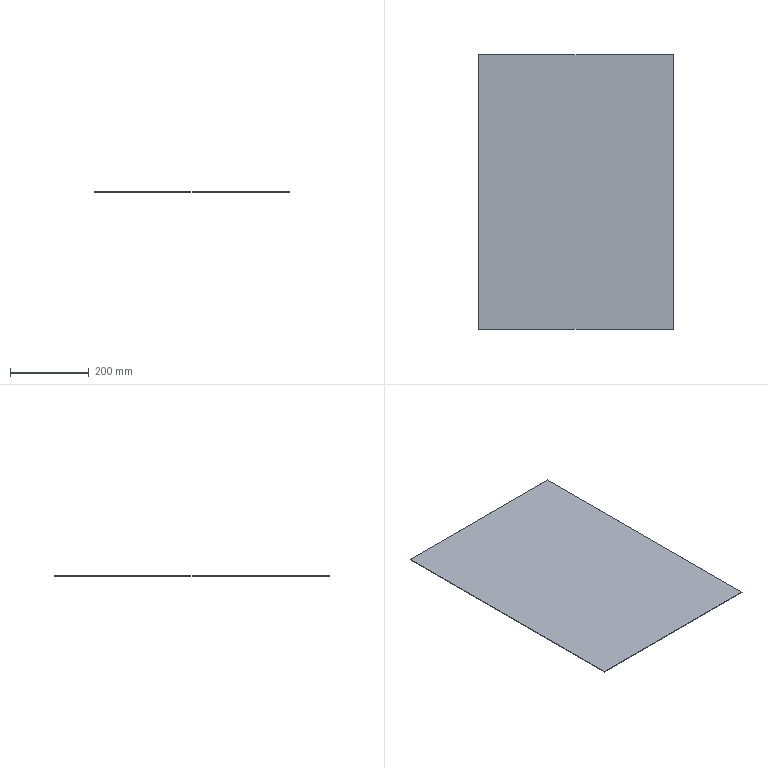Part | SolidWorks | 1 solid | 6 faces | box 496 x 700 x 1.5 mm | volume 520800 mm3 | plane 6
STEP:
#1=CARTESIAN_POINT('',(248.,-350.,0.));
#2=VERTEX_POINT('',#1);
#3=CARTESIAN_POINT('',(248.,350.,0.));
#4=VERTEX_POINT('',#3);
#5=CARTESIAN_POINT('',(248.,-350.,0.));
#6=DIRECTION('',(0.,1.,0.));
#7=VECTOR('',#6,1000.);
#8=LINE('',#5,#7);
#9=EDGE_CURVE('',#2,#4,#8,.T.);
#10=ORIENTED_EDGE('',*,*,#9,.T.);
#11=CARTESIAN_POINT('',(248.,350.,1.5));
#12=VERTEX_POINT('',#11);
#13=CARTESIAN_POINT('',(248.,350.,1.5));
#14=DIRECTION('',(0.,0.,-1.));
#15=VECTOR('',#14,1000.);
#16=LINE('',#13,#15);
#17=EDGE_CURVE('',#12,#4,#16,.T.);
#18=ORIENTED_EDGE('',*,*,#17,.F.);
#19=CARTESIAN_POINT('',(248.,-350.,1.5));
#20=VERTEX_POINT('',#19);
#21=CARTESIAN_POINT('',(248.,-350.,1.5));
#22=DIRECTION('',(0.,1.,0.));
#23=VECTOR('',#22,1000.);
#24=LINE('',#21,#23);
#25=EDGE_CURVE('',#20,#12,#24,.T.);
#26=ORIENTED_EDGE('',*,*,#25,.F.);
#27=CARTESIAN_POINT('',(248.,-350.,1.5));
#28=DIRECTION('',(0.,0.,-1.));
#29=VECTOR('',#28,1000.);
#30=LINE('',#27,#29);
#31=EDGE_CURVE('',#20,#2,#30,.T.);
#32=ORIENTED_EDGE('',*,*,#31,.T.);
#33=EDGE_LOOP('',(#10,#18,#26,#32));
#34=FACE_OUTER_BOUND('',#33,.T.);
#35=CARTESIAN_POINT('',(248.,-350.,1.5));
#36=DIRECTION('',(-1.,0.,0.));
#37=DIRECTION('',(0.,0.,1.));
#38=AXIS2_PLACEMENT_3D('',#35,#36,#37);
#39=PLANE('',#38);
#40=ADVANCED_FACE('',(#34),#39,.F.);
#41=CARTESIAN_POINT('',(-248.,350.,0.));
#42=VERTEX_POINT('',#41);
#43=CARTESIAN_POINT('',(248.,350.,0.));
#44=DIRECTION('',(-1.,0.,0.));
#45=VECTOR('',#44,1000.);
#46=LINE('',#43,#45);
#47=EDGE_CURVE('',#4,#42,#46,.T.);
#48=ORIENTED_EDGE('',*,*,#47,.T.);
#49=CARTESIAN_POINT('',(-248.,350.,1.5));
#50=VERTEX_POINT('',#49);
#51=CARTESIAN_POINT('',(-248.,350.,1.5));
#52=DIRECTION('',(0.,0.,-1.));
#53=VECTOR('',#52,1000.);
#54=LINE('',#51,#53);
#55=EDGE_CURVE('',#50,#42,#54,.T.);
#56=ORIENTED_EDGE('',*,*,#55,.F.);
#57=CARTESIAN_POINT('',(248.,350.,1.5));
#58=DIRECTION('',(-1.,0.,0.));
#59=VECTOR('',#58,1000.);
#60=LINE('',#57,#59);
#61=EDGE_CURVE('',#12,#50,#60,.T.);
#62=ORIENTED_EDGE('',*,*,#61,.F.);
#63=ORIENTED_EDGE('',*,*,#17,.T.);
#64=EDGE_LOOP('',(#48,#56,#62,#63));
#65=FACE_OUTER_BOUND('',#64,.T.);
#66=CARTESIAN_POINT('',(248.,350.,1.5));
#67=DIRECTION('',(0.,-1.,0.));
#68=DIRECTION('',(0.,0.,-1.));
#69=AXIS2_PLACEMENT_3D('',#66,#67,#68);
#70=PLANE('',#69);
#71=ADVANCED_FACE('',(#65),#70,.F.);
#72=CARTESIAN_POINT('',(-248.,-350.,0.));
#73=VERTEX_POINT('',#72);
#74=CARTESIAN_POINT('',(-248.,-350.,0.));
#75=DIRECTION('',(0.,-1.,0.));
#76=VECTOR('',#75,1000.);
#77=LINE('',#74,#76);
#78=EDGE_CURVE('',#42,#73,#77,.T.);
#79=ORIENTED_EDGE('',*,*,#78,.T.);
#80=CARTESIAN_POINT('',(-248.,-350.,1.5));
#81=VERTEX_POINT('',#80);
#82=CARTESIAN_POINT('',(-248.,-350.,1.5));
#83=DIRECTION('',(0.,0.,-1.));
#84=VECTOR('',#83,1000.);
#85=LINE('',#82,#84);
#86=EDGE_CURVE('',#81,#73,#85,.T.);
#87=ORIENTED_EDGE('',*,*,#86,.F.);
#88=CARTESIAN_POINT('',(-248.,-350.,1.5));
#89=DIRECTION('',(0.,-1.,0.));
#90=VECTOR('',#89,1000.);
#91=LINE('',#88,#90);
#92=EDGE_CURVE('',#50,#81,#91,.T.);
#93=ORIENTED_EDGE('',*,*,#92,.F.);
#94=ORIENTED_EDGE('',*,*,#55,.T.);
#95=EDGE_LOOP('',(#79,#87,#93,#94));
#96=FACE_OUTER_BOUND('',#95,.T.);
#97=CARTESIAN_POINT('',(-248.,-350.,1.5));
#98=DIRECTION('',(1.,0.,0.));
#99=DIRECTION('',(0.,0.,-1.));
#100=AXIS2_PLACEMENT_3D('',#97,#98,#99);
#101=PLANE('',#100);
#102=ADVANCED_FACE('',(#96),#101,.F.);
#103=CARTESIAN_POINT('',(248.,-350.,0.));
#104=DIRECTION('',(1.,0.,0.));
#105=VECTOR('',#104,1000.);
#106=LINE('',#103,#105);
#107=EDGE_CURVE('',#73,#2,#106,.T.);
#108=ORIENTED_EDGE('',*,*,#107,.T.);
#109=ORIENTED_EDGE('',*,*,#31,.F.);
#110=CARTESIAN_POINT('',(248.,-350.,1.5));
#111=DIRECTION('',(1.,0.,0.));
#112=VECTOR('',#111,1000.);
#113=LINE('',#110,#112);
#114=EDGE_CURVE('',#81,#20,#113,.T.);
#115=ORIENTED_EDGE('',*,*,#114,.F.);
#116=ORIENTED_EDGE('',*,*,#86,.T.);
#117=EDGE_LOOP('',(#108,#109,#115,#116));
#118=FACE_OUTER_BOUND('',#117,.T.);
#119=CARTESIAN_POINT('',(248.,-350.,1.5));
#120=DIRECTION('',(0.,1.,0.));
#121=DIRECTION('',(0.,0.,1.));
#122=AXIS2_PLACEMENT_3D('',#119,#120,#121);
#123=PLANE('',#122);
#124=ADVANCED_FACE('',(#118),#123,.F.);
#125=ORIENTED_EDGE('',*,*,#25,.T.);
#126=ORIENTED_EDGE('',*,*,#61,.T.);
#127=ORIENTED_EDGE('',*,*,#92,.T.);
#128=ORIENTED_EDGE('',*,*,#114,.T.);
#129=EDGE_LOOP('',(#125,#126,#127,#128));
#130=FACE_OUTER_BOUND('',#129,.T.);
#131=CARTESIAN_POINT('',(0.,0.,1.5));
#132=DIRECTION('',(0.,0.,1.));
#133=DIRECTION('',(1.,0.,0.));
#134=AXIS2_PLACEMENT_3D('',#131,#132,#133);
#135=PLANE('',#134);
#136=ADVANCED_FACE('',(#130),#135,.T.);
#137=ORIENTED_EDGE('',*,*,#9,.F.);
#138=ORIENTED_EDGE('',*,*,#107,.F.);
#139=ORIENTED_EDGE('',*,*,#78,.F.);
#140=ORIENTED_EDGE('',*,*,#47,.F.);
#141=EDGE_LOOP('',(#137,#138,#139,#140));
#142=FACE_OUTER_BOUND('',#141,.T.);
#143=CARTESIAN_POINT('',(0.,0.,0.));
#144=DIRECTION('',(0.,0.,1.));
#145=DIRECTION('',(1.,0.,0.));
#146=AXIS2_PLACEMENT_3D('',#143,#144,#145);
#147=PLANE('',#146);
#148=ADVANCED_FACE('',(#142),#147,.F.);
#149=CLOSED_SHELL('',(#40,#71,#102,#124,#136,#148));
#150=MANIFOLD_SOLID_BREP('',#149);
#151=CARTESIAN_POINT('',(0.,0.,0.));
#152=DIRECTION('',(0.,0.,1.));
#153=DIRECTION('',(1.,0.,0.));
#154=AXIS2_PLACEMENT_3D('',#151,#152,#153);
#155=(LENGTH_UNIT()NAMED_UNIT(*)SI_UNIT(.MILLI.,.METRE.));
#156=UNCERTAINTY_MEASURE_WITH_UNIT(LENGTH_MEASURE(0.00001),#155,'','');
#157=(NAMED_UNIT(*)PLANE_ANGLE_UNIT()SI_UNIT($,.RADIAN.));
#158=(NAMED_UNIT(*)SI_UNIT($,.STERADIAN.)SOLID_ANGLE_UNIT());
#159=(GEOMETRIC_REPRESENTATION_CONTEXT(3)GLOBAL_UNCERTAINTY_ASSIGNED_CONTEXT((#156))GLOBAL_UNIT_ASSIGNED_CONTEXT((#155,#157,#158))REPRESENTATION_CONTEXT('',''));
#160=ADVANCED_BREP_SHAPE_REPRESENTATION('',(#150,#154),#159);